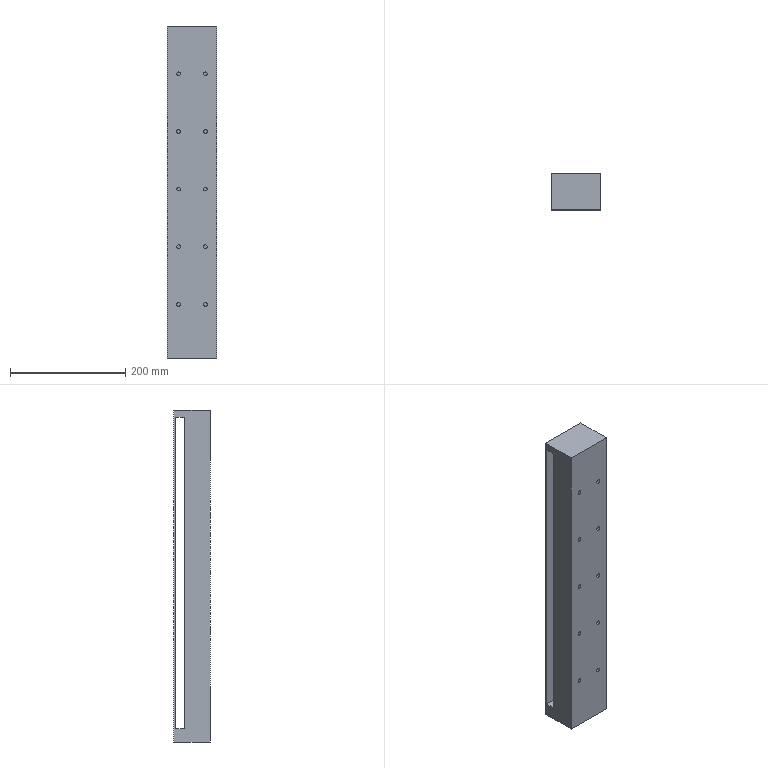Part | SolidWorks | features BaseBody 1 | 1 solid | 34 faces | box 86 x 63 x 576 mm | volume 613007 mm3 | cylinder 20 | plane 14 | commonest cylinder face diameters 6.5 x20
STEP:
#1=CARTESIAN_POINT('',(23.,-148.847,202.371));
#2=VERTEX_POINT('',#1);
#3=CARTESIAN_POINT('',(23.,-148.847,195.871));
#4=VERTEX_POINT('',#3);
#5=CARTESIAN_POINT('',(23.,-148.847,199.121));
#6=DIRECTION('',(0.,-1.,0.));
#7=DIRECTION('',(0.,0.,-1.));
#8=AXIS2_PLACEMENT_3D('',#5,#6,#7);
#9=CIRCLE('',#8,3.25);
#10=EDGE_CURVE('',#2,#4,#9,.T.);
#11=ORIENTED_EDGE('',*,*,#10,.F.);
#12=CARTESIAN_POINT('',(23.,-153.,202.371));
#13=VERTEX_POINT('',#12);
#14=CARTESIAN_POINT('',(23.,-133.,202.371));
#15=DIRECTION('',(0.,-1.,0.));
#16=VECTOR('',#15,1000.);
#17=LINE('',#14,#16);
#18=EDGE_CURVE('',#2,#13,#17,.T.);
#19=ORIENTED_EDGE('',*,*,#18,.T.);
#20=CARTESIAN_POINT('',(23.,-153.,195.871));
#21=VERTEX_POINT('',#20);
#22=CARTESIAN_POINT('',(23.,-153.,199.121));
#23=DIRECTION('',(0.,-1.,0.));
#24=DIRECTION('',(0.,0.,-1.));
#25=AXIS2_PLACEMENT_3D('',#22,#23,#24);
#26=CIRCLE('',#25,3.25);
#27=EDGE_CURVE('',#13,#21,#26,.T.);
#28=ORIENTED_EDGE('',*,*,#27,.T.);
#29=CARTESIAN_POINT('',(23.,-133.,195.871));
#30=DIRECTION('',(0.,-1.,0.));
#31=VECTOR('',#30,1000.);
#32=LINE('',#29,#31);
#33=EDGE_CURVE('',#4,#21,#32,.T.);
#34=ORIENTED_EDGE('',*,*,#33,.F.);
#35=EDGE_LOOP('',(#11,#19,#28,#34));
#36=FACE_OUTER_BOUND('',#35,.T.);
#37=CARTESIAN_POINT('',(23.,-133.,199.121));
#38=DIRECTION('',(0.,-1.,0.));
#39=DIRECTION('',(0.,0.,-1.));
#40=AXIS2_PLACEMENT_3D('',#37,#38,#39);
#41=CYLINDRICAL_SURFACE('',#40,3.25);
#42=ADVANCED_FACE('',(#36),#41,.F.);
#43=CARTESIAN_POINT('',(-23.,-148.847,202.371));
#44=VERTEX_POINT('',#43);
#45=CARTESIAN_POINT('',(-23.,-148.847,195.871));
#46=VERTEX_POINT('',#45);
#47=CARTESIAN_POINT('',(-23.,-148.847,199.121));
#48=DIRECTION('',(0.,-1.,0.));
#49=DIRECTION('',(0.,0.,-1.));
#50=AXIS2_PLACEMENT_3D('',#47,#48,#49);
#51=CIRCLE('',#50,3.25);
#52=EDGE_CURVE('',#44,#46,#51,.T.);
#53=ORIENTED_EDGE('',*,*,#52,.F.);
#54=CARTESIAN_POINT('',(-23.,-153.,202.371));
#55=VERTEX_POINT('',#54);
#56=CARTESIAN_POINT('',(-23.,-133.,202.371));
#57=DIRECTION('',(0.,-1.,0.));
#58=VECTOR('',#57,1000.);
#59=LINE('',#56,#58);
#60=EDGE_CURVE('',#44,#55,#59,.T.);
#61=ORIENTED_EDGE('',*,*,#60,.T.);
#62=CARTESIAN_POINT('',(-23.,-153.,195.871));
#63=VERTEX_POINT('',#62);
#64=CARTESIAN_POINT('',(-23.,-153.,199.121));
#65=DIRECTION('',(0.,-1.,0.));
#66=DIRECTION('',(0.,0.,-1.));
#67=AXIS2_PLACEMENT_3D('',#64,#65,#66);
#68=CIRCLE('',#67,3.25);
#69=EDGE_CURVE('',#55,#63,#68,.T.);
#70=ORIENTED_EDGE('',*,*,#69,.T.);
#71=CARTESIAN_POINT('',(-23.,-133.,195.871));
#72=DIRECTION('',(0.,-1.,0.));
#73=VECTOR('',#72,1000.);
#74=LINE('',#71,#73);
#75=EDGE_CURVE('',#46,#63,#74,.T.);
#76=ORIENTED_EDGE('',*,*,#75,.F.);
#77=EDGE_LOOP('',(#53,#61,#70,#76));
#78=FACE_OUTER_BOUND('',#77,.T.);
#79=CARTESIAN_POINT('',(-23.,-133.,199.121));
#80=DIRECTION('',(0.,-1.,0.));
#81=DIRECTION('',(0.,0.,-1.));
#82=AXIS2_PLACEMENT_3D('',#79,#80,#81);
#83=CYLINDRICAL_SURFACE('',#82,3.25);
#84=ADVANCED_FACE('',(#78),#83,.F.);
#85=CARTESIAN_POINT('',(23.,-148.847,102.371));
#86=VERTEX_POINT('',#85);
#87=CARTESIAN_POINT('',(23.,-148.847,95.871));
#88=VERTEX_POINT('',#87);
#89=CARTESIAN_POINT('',(23.,-148.847,99.121));
#90=DIRECTION('',(0.,-1.,0.));
#91=DIRECTION('',(0.,0.,-1.));
#92=AXIS2_PLACEMENT_3D('',#89,#90,#91);
#93=CIRCLE('',#92,3.25);
#94=EDGE_CURVE('',#86,#88,#93,.T.);
#95=ORIENTED_EDGE('',*,*,#94,.F.);
#96=CARTESIAN_POINT('',(23.,-153.,102.371));
#97=VERTEX_POINT('',#96);
#98=CARTESIAN_POINT('',(23.,-133.,102.371));
#99=DIRECTION('',(0.,-1.,0.));
#100=VECTOR('',#99,1000.);
#101=LINE('',#98,#100);
#102=EDGE_CURVE('',#86,#97,#101,.T.);
#103=ORIENTED_EDGE('',*,*,#102,.T.);
#104=CARTESIAN_POINT('',(23.,-153.,95.871));
#105=VERTEX_POINT('',#104);
#106=CARTESIAN_POINT('',(23.,-153.,99.121));
#107=DIRECTION('',(0.,-1.,0.));
#108=DIRECTION('',(0.,0.,-1.));
#109=AXIS2_PLACEMENT_3D('',#106,#107,#108);
#110=CIRCLE('',#109,3.25);
#111=EDGE_CURVE('',#97,#105,#110,.T.);
#112=ORIENTED_EDGE('',*,*,#111,.T.);
#113=CARTESIAN_POINT('',(23.,-133.,95.871));
#114=DIRECTION('',(0.,-1.,0.));
#115=VECTOR('',#114,1000.);
#116=LINE('',#113,#115);
#117=EDGE_CURVE('',#88,#105,#116,.T.);
#118=ORIENTED_EDGE('',*,*,#117,.F.);
#119=EDGE_LOOP('',(#95,#103,#112,#118));
#120=FACE_OUTER_BOUND('',#119,.T.);
#121=CARTESIAN_POINT('',(23.,-133.,99.121));
#122=DIRECTION('',(0.,-1.,0.));
#123=DIRECTION('',(0.,0.,-1.));
#124=AXIS2_PLACEMENT_3D('',#121,#122,#123);
#125=CYLINDRICAL_SURFACE('',#124,3.25);
#126=ADVANCED_FACE('',(#120),#125,.F.);
#127=CARTESIAN_POINT('',(-23.,-148.847,102.371));
#128=VERTEX_POINT('',#127);
#129=CARTESIAN_POINT('',(-23.,-148.847,95.871));
#130=VERTEX_POINT('',#129);
#131=CARTESIAN_POINT('',(-23.,-148.847,99.121));
#132=DIRECTION('',(0.,-1.,0.));
#133=DIRECTION('',(0.,0.,-1.));
#134=AXIS2_PLACEMENT_3D('',#131,#132,#133);
#135=CIRCLE('',#134,3.25);
#136=EDGE_CURVE('',#128,#130,#135,.T.);
#137=ORIENTED_EDGE('',*,*,#136,.F.);
#138=CARTESIAN_POINT('',(-23.,-153.,102.371));
#139=VERTEX_POINT('',#138);
#140=CARTESIAN_POINT('',(-23.,-133.,102.371));
#141=DIRECTION('',(0.,-1.,0.));
#142=VECTOR('',#141,1000.);
#143=LINE('',#140,#142);
#144=EDGE_CURVE('',#128,#139,#143,.T.);
#145=ORIENTED_EDGE('',*,*,#144,.T.);
#146=CARTESIAN_POINT('',(-23.,-153.,95.871));
#147=VERTEX_POINT('',#146);
#148=CARTESIAN_POINT('',(-23.,-153.,99.121));
#149=DIRECTION('',(0.,-1.,0.));
#150=DIRECTION('',(0.,0.,-1.));
#151=AXIS2_PLACEMENT_3D('',#148,#149,#150);
#152=CIRCLE('',#151,3.25);
#153=EDGE_CURVE('',#139,#147,#152,.T.);
#154=ORIENTED_EDGE('',*,*,#153,.T.);
#155=CARTESIAN_POINT('',(-23.,-133.,95.871));
#156=DIRECTION('',(0.,-1.,0.));
#157=VECTOR('',#156,1000.);
#158=LINE('',#155,#157);
#159=EDGE_CURVE('',#130,#147,#158,.T.);
#160=ORIENTED_EDGE('',*,*,#159,.F.);
#161=EDGE_LOOP('',(#137,#145,#154,#160));
#162=FACE_OUTER_BOUND('',#161,.T.);
#163=CARTESIAN_POINT('',(-23.,-133.,99.121));
#164=DIRECTION('',(0.,-1.,0.));
#165=DIRECTION('',(0.,0.,-1.));
#166=AXIS2_PLACEMENT_3D('',#163,#164,#165);
#167=CYLINDRICAL_SURFACE('',#166,3.25);
#168=ADVANCED_FACE('',(#162),#167,.F.);
#169=CARTESIAN_POINT('',(23.,-148.847,2.371));
#170=VERTEX_POINT('',#169);
#171=CARTESIAN_POINT('',(23.,-148.847,-4.129));
#172=VERTEX_POINT('',#171);
#173=CARTESIAN_POINT('',(23.,-148.847,-0.8789));
#174=DIRECTION('',(0.,-1.,0.));
#175=DIRECTION('',(0.,0.,-1.));
#176=AXIS2_PLACEMENT_3D('',#173,#174,#175);
#177=CIRCLE('',#176,3.25);
#178=EDGE_CURVE('',#170,#172,#177,.T.);
#179=ORIENTED_EDGE('',*,*,#178,.F.);
#180=CARTESIAN_POINT('',(23.,-153.,2.371));
#181=VERTEX_POINT('',#180);
#182=CARTESIAN_POINT('',(23.,-133.,2.371));
#183=DIRECTION('',(0.,-1.,0.));
#184=VECTOR('',#183,1000.);
#185=LINE('',#182,#184);
#186=EDGE_CURVE('',#170,#181,#185,.T.);
#187=ORIENTED_EDGE('',*,*,#186,.T.);
#188=CARTESIAN_POINT('',(23.,-153.,-4.129));
#189=VERTEX_POINT('',#188);
#190=CARTESIAN_POINT('',(23.,-153.,-0.8789));
#191=DIRECTION('',(0.,-1.,0.));
#192=DIRECTION('',(0.,0.,-1.));
#193=AXIS2_PLACEMENT_3D('',#190,#191,#192);
#194=CIRCLE('',#193,3.25);
#195=EDGE_CURVE('',#181,#189,#194,.T.);
#196=ORIENTED_EDGE('',*,*,#195,.T.);
#197=CARTESIAN_POINT('',(23.,-133.,-4.129));
#198=DIRECTION('',(0.,-1.,0.));
#199=VECTOR('',#198,1000.);
#200=LINE('',#197,#199);
#201=EDGE_CURVE('',#172,#189,#200,.T.);
#202=ORIENTED_EDGE('',*,*,#201,.F.);
#203=EDGE_LOOP('',(#179,#187,#196,#202));
#204=FACE_OUTER_BOUND('',#203,.T.);
#205=CARTESIAN_POINT('',(23.,-133.,-0.8789));
#206=DIRECTION('',(0.,-1.,0.));
#207=DIRECTION('',(0.,0.,-1.));
#208=AXIS2_PLACEMENT_3D('',#205,#206,#207);
#209=CYLINDRICAL_SURFACE('',#208,3.25);
#210=ADVANCED_FACE('',(#204),#209,.F.);
#211=CARTESIAN_POINT('',(-23.,-148.847,2.371));
#212=VERTEX_POINT('',#211);
#213=CARTESIAN_POINT('',(-23.,-148.847,-4.129));
#214=VERTEX_POINT('',#213);
#215=CARTESIAN_POINT('',(-23.,-148.847,-0.8789));
#216=DIRECTION('',(0.,-1.,0.));
#217=DIRECTION('',(0.,0.,-1.));
#218=AXIS2_PLACEMENT_3D('',#215,#216,#217);
#219=CIRCLE('',#218,3.25);
#220=EDGE_CURVE('',#212,#214,#219,.T.);
#221=ORIENTED_EDGE('',*,*,#220,.F.);
#222=CARTESIAN_POINT('',(-23.,-153.,2.371));
#223=VERTEX_POINT('',#222);
#224=CARTESIAN_POINT('',(-23.,-133.,2.371));
#225=DIRECTION('',(0.,-1.,0.));
#226=VECTOR('',#225,1000.);
#227=LINE('',#224,#226);
#228=EDGE_CURVE('',#212,#223,#227,.T.);
#229=ORIENTED_EDGE('',*,*,#228,.T.);
#230=CARTESIAN_POINT('',(-23.,-153.,-4.129));
#231=VERTEX_POINT('',#230);
#232=CARTESIAN_POINT('',(-23.,-153.,-0.8789));
#233=DIRECTION('',(0.,-1.,0.));
#234=DIRECTION('',(0.,0.,-1.));
#235=AXIS2_PLACEMENT_3D('',#232,#233,#234);
#236=CIRCLE('',#235,3.25);
#237=EDGE_CURVE('',#223,#231,#236,.T.);
#238=ORIENTED_EDGE('',*,*,#237,.T.);
#239=CARTESIAN_POINT('',(-23.,-133.,-4.129));
#240=DIRECTION('',(0.,-1.,0.));
#241=VECTOR('',#240,1000.);
#242=LINE('',#239,#241);
#243=EDGE_CURVE('',#214,#231,#242,.T.);
#244=ORIENTED_EDGE('',*,*,#243,.F.);
#245=EDGE_LOOP('',(#221,#229,#238,#244));
#246=FACE_OUTER_BOUND('',#245,.T.);
#247=CARTESIAN_POINT('',(-23.,-133.,-0.8789));
#248=DIRECTION('',(0.,-1.,0.));
#249=DIRECTION('',(0.,0.,-1.));
#250=AXIS2_PLACEMENT_3D('',#247,#248,#249);
#251=CYLINDRICAL_SURFACE('',#250,3.25);
#252=ADVANCED_FACE('',(#246),#251,.F.);
#253=CARTESIAN_POINT('',(23.,-148.847,-97.629));
#254=VERTEX_POINT('',#253);
#255=CARTESIAN_POINT('',(23.,-148.847,-104.129));
#256=VERTEX_POINT('',#255);
#257=CARTESIAN_POINT('',(23.,-148.847,-100.879));
#258=DIRECTION('',(0.,-1.,0.));
#259=DIRECTION('',(0.,0.,-1.));
#260=AXIS2_PLACEMENT_3D('',#257,#258,#259);
#261=CIRCLE('',#260,3.25);
#262=EDGE_CURVE('',#254,#256,#261,.T.);
#263=ORIENTED_EDGE('',*,*,#262,.F.);
#264=CARTESIAN_POINT('',(23.,-153.,-97.629));
#265=VERTEX_POINT('',#264);
#266=CARTESIAN_POINT('',(23.,-133.,-97.629));
#267=DIRECTION('',(0.,-1.,0.));
#268=VECTOR('',#267,1000.);
#269=LINE('',#266,#268);
#270=EDGE_CURVE('',#254,#265,#269,.T.);
#271=ORIENTED_EDGE('',*,*,#270,.T.);
#272=CARTESIAN_POINT('',(23.,-153.,-104.129));
#273=VERTEX_POINT('',#272);
#274=CARTESIAN_POINT('',(23.,-153.,-100.879));
#275=DIRECTION('',(0.,-1.,0.));
#276=DIRECTION('',(0.,0.,-1.));
#277=AXIS2_PLACEMENT_3D('',#274,#275,#276);
#278=CIRCLE('',#277,3.25);
#279=EDGE_CURVE('',#265,#273,#278,.T.);
#280=ORIENTED_EDGE('',*,*,#279,.T.);
#281=CARTESIAN_POINT('',(23.,-133.,-104.129));
#282=DIRECTION('',(0.,-1.,0.));
#283=VECTOR('',#282,1000.);
#284=LINE('',#281,#283);
#285=EDGE_CURVE('',#256,#273,#284,.T.);
#286=ORIENTED_EDGE('',*,*,#285,.F.);
#287=EDGE_LOOP('',(#263,#271,#280,#286));
#288=FACE_OUTER_BOUND('',#287,.T.);
#289=CARTESIAN_POINT('',(23.,-133.,-100.879));
#290=DIRECTION('',(0.,-1.,0.));
#291=DIRECTION('',(0.,0.,-1.));
#292=AXIS2_PLACEMENT_3D('',#289,#290,#291);
#293=CYLINDRICAL_SURFACE('',#292,3.25);
#294=ADVANCED_FACE('',(#288),#293,.F.);
#295=CARTESIAN_POINT('',(-23.,-148.847,-97.629));
#296=VERTEX_POINT('',#295);
#297=CARTESIAN_POINT('',(-23.,-148.847,-104.129));
#298=VERTEX_POINT('',#297);
#299=CARTESIAN_POINT('',(-23.,-148.847,-100.879));
#300=DIRECTION('',(0.,-1.,0.));
#301=DIRECTION('',(0.,0.,-1.));
#302=AXIS2_PLACEMENT_3D('',#299,#300,#301);
#303=CIRCLE('',#302,3.25);
#304=EDGE_CURVE('',#296,#298,#303,.T.);
#305=ORIENTED_EDGE('',*,*,#304,.F.);
#306=CARTESIAN_POINT('',(-23.,-153.,-97.629));
#307=VERTEX_POINT('',#306);
#308=CARTESIAN_POINT('',(-23.,-133.,-97.629));
#309=DIRECTION('',(0.,-1.,0.));
#310=VECTOR('',#309,1000.);
#311=LINE('',#308,#310);
#312=EDGE_CURVE('',#296,#307,#311,.T.);
#313=ORIENTED_EDGE('',*,*,#312,.T.);
#314=CARTESIAN_POINT('',(-23.,-153.,-104.129));
#315=VERTEX_POINT('',#314);
#316=CARTESIAN_POINT('',(-23.,-153.,-100.879));
#317=DIRECTION('',(0.,-1.,0.));
#318=DIRECTION('',(0.,0.,-1.));
#319=AXIS2_PLACEMENT_3D('',#316,#317,#318);
#320=CIRCLE('',#319,3.25);
#321=EDGE_CURVE('',#307,#315,#320,.T.);
#322=ORIENTED_EDGE('',*,*,#321,.T.);
#323=CARTESIAN_POINT('',(-23.,-133.,-104.129));
#324=DIRECTION('',(0.,-1.,0.));
#325=VECTOR('',#324,1000.);
#326=LINE('',#323,#325);
#327=EDGE_CURVE('',#298,#315,#326,.T.);
#328=ORIENTED_EDGE('',*,*,#327,.F.);
#329=EDGE_LOOP('',(#305,#313,#322,#328));
#330=FACE_OUTER_BOUND('',#329,.T.);
#331=CARTESIAN_POINT('',(-23.,-133.,-100.879));
#332=DIRECTION('',(0.,-1.,0.));
#333=DIRECTION('',(0.,0.,-1.));
#334=AXIS2_PLACEMENT_3D('',#331,#332,#333);
#335=CYLINDRICAL_SURFACE('',#334,3.25);
#336=ADVANCED_FACE('',(#330),#335,.F.);
#337=CARTESIAN_POINT('',(23.,-148.847,-197.629));
#338=VERTEX_POINT('',#337);
#339=CARTESIAN_POINT('',(23.,-148.847,-204.129));
#340=VERTEX_POINT('',#339);
#341=CARTESIAN_POINT('',(23.,-148.847,-200.879));
#342=DIRECTION('',(0.,-1.,0.));
#343=DIRECTION('',(0.,0.,-1.));
#344=AXIS2_PLACEMENT_3D('',#341,#342,#343);
#345=CIRCLE('',#344,3.25);
#346=EDGE_CURVE('',#338,#340,#345,.T.);
#347=ORIENTED_EDGE('',*,*,#346,.F.);
#348=CARTESIAN_POINT('',(23.,-153.,-197.629));
#349=VERTEX_POINT('',#348);
#350=CARTESIAN_POINT('',(23.,-133.,-197.629));
#351=DIRECTION('',(0.,-1.,0.));
#352=VECTOR('',#351,1000.);
#353=LINE('',#350,#352);
#354=EDGE_CURVE('',#338,#349,#353,.T.);
#355=ORIENTED_EDGE('',*,*,#354,.T.);
#356=CARTESIAN_POINT('',(23.,-153.,-204.129));
#357=VERTEX_POINT('',#356);
#358=CARTESIAN_POINT('',(23.,-153.,-200.879));
#359=DIRECTION('',(0.,-1.,0.));
#360=DIRECTION('',(0.,0.,-1.));
#361=AXIS2_PLACEMENT_3D('',#358,#359,#360);
#362=CIRCLE('',#361,3.25);
#363=EDGE_CURVE('',#349,#357,#362,.T.);
#364=ORIENTED_EDGE('',*,*,#363,.T.);
#365=CARTESIAN_POINT('',(23.,-133.,-204.129));
#366=DIRECTION('',(0.,-1.,0.));
#367=VECTOR('',#366,1000.);
#368=LINE('',#365,#367);
#369=EDGE_CURVE('',#340,#357,#368,.T.);
#370=ORIENTED_EDGE('',*,*,#369,.F.);
#371=EDGE_LOOP('',(#347,#355,#364,#370));
#372=FACE_OUTER_BOUND('',#371,.T.);
#373=CARTESIAN_POINT('',(23.,-133.,-200.879));
#374=DIRECTION('',(0.,-1.,0.));
#375=DIRECTION('',(0.,0.,-1.));
#376=AXIS2_PLACEMENT_3D('',#373,#374,#375);
#377=CYLINDRICAL_SURFACE('',#376,3.25);
#378=ADVANCED_FACE('',(#372),#377,.F.);
#379=CARTESIAN_POINT('',(-23.,-148.847,-197.629));
#380=VERTEX_POINT('',#379);
#381=CARTESIAN_POINT('',(-23.,-148.847,-204.129));
#382=VERTEX_POINT('',#381);
#383=CARTESIAN_POINT('',(-23.,-148.847,-200.879));
#384=DIRECTION('',(0.,-1.,0.));
#385=DIRECTION('',(0.,0.,-1.));
#386=AXIS2_PLACEMENT_3D('',#383,#384,#385);
#387=CIRCLE('',#386,3.25);
#388=EDGE_CURVE('',#380,#382,#387,.T.);
#389=ORIENTED_EDGE('',*,*,#388,.F.);
#390=CARTESIAN_POINT('',(-23.,-153.,-197.629));
#391=VERTEX_POINT('',#390);
#392=CARTESIAN_POINT('',(-23.,-133.,-197.629));
#393=DIRECTION('',(0.,-1.,0.));
#394=VECTOR('',#393,1000.);
#395=LINE('',#392,#394);
#396=EDGE_CURVE('',#380,#391,#395,.T.);
#397=ORIENTED_EDGE('',*,*,#396,.T.);
#398=CARTESIAN_POINT('',(-23.,-153.,-204.129));
#399=VERTEX_POINT('',#398);
#400=CARTESIAN_POINT('',(-23.,-153.,-200.879));
#401=DIRECTION('',(0.,-1.,0.));
#402=DIRECTION('',(0.,0.,-1.));
#403=AXIS2_PLACEMENT_3D('',#400,#401,#402);
#404=CIRCLE('',#403,3.25);
#405=EDGE_CURVE('',#391,#399,#404,.T.);
#406=ORIENTED_EDGE('',*,*,#405,.T.);
#407=CARTESIAN_POINT('',(-23.,-133.,-204.129));
#408=DIRECTION('',(0.,-1.,0.));
#409=VECTOR('',#408,1000.);
#410=LINE('',#407,#409);
#411=EDGE_CURVE('',#382,#399,#410,.T.);
#412=ORIENTED_EDGE('',*,*,#411,.F.);
#413=EDGE_LOOP('',(#389,#397,#406,#412));
#414=FACE_OUTER_BOUND('',#413,.T.);
#415=CARTESIAN_POINT('',(-23.,-133.,-200.879));
#416=DIRECTION('',(0.,-1.,0.));
#417=DIRECTION('',(0.,0.,-1.));
#418=AXIS2_PLACEMENT_3D('',#415,#416,#417);
#419=CYLINDRICAL_SURFACE('',#418,3.25);
#420=ADVANCED_FACE('',(#414),#419,.F.);
#421=CARTESIAN_POINT('',(-43.,-90.,282.121));
#422=VERTEX_POINT('',#421);
#423=CARTESIAN_POINT('',(-43.,-90.,-293.879));
#424=VERTEX_POINT('',#423);
#425=CARTESIAN_POINT('',(-43.,-90.,282.121));
#426=DIRECTION('',(0.,0.,-1.));
#427=VECTOR('',#426,1000.);
#428=LINE('',#425,#427);
#429=EDGE_CURVE('',#422,#424,#428,.T.);
#430=ORIENTED_EDGE('',*,*,#429,.F.);
#431=CARTESIAN_POINT('',(43.,-90.,282.121));
#432=VERTEX_POINT('',#431);
#433=CARTESIAN_POINT('',(-43.,-90.,282.121));
#434=DIRECTION('',(-1.,0.,0.));
#435=VECTOR('',#434,1000.);
#436=LINE('',#433,#435);
#437=EDGE_CURVE('',#432,#422,#436,.T.);
#438=ORIENTED_EDGE('',*,*,#437,.F.);
#439=CARTESIAN_POINT('',(43.,-90.,-293.879));
#440=VERTEX_POINT('',#439);
#441=CARTESIAN_POINT('',(43.,-90.,282.121));
#442=DIRECTION('',(0.,0.,1.));
#443=VECTOR('',#442,1000.);
#444=LINE('',#441,#443);
#445=EDGE_CURVE('',#440,#432,#444,.T.);
#446=ORIENTED_EDGE('',*,*,#445,.F.);
#447=CARTESIAN_POINT('',(-43.,-90.,-293.879));
#448=DIRECTION('',(1.,0.,0.));
#449=VECTOR('',#448,1000.);
#450=LINE('',#447,#449);
#451=EDGE_CURVE('',#424,#440,#450,.T.);
#452=ORIENTED_EDGE('',*,*,#451,.F.);
#453=EDGE_LOOP('',(#430,#438,#446,#452));
#454=FACE_OUTER_BOUND('',#453,.T.);
#455=CARTESIAN_POINT('',(-43.,-90.,282.121));
#456=DIRECTION('',(0.,-1.,0.));
#457=DIRECTION('',(0.,0.,-1.));
#458=AXIS2_PLACEMENT_3D('',#455,#456,#457);
#459=PLANE('',#458);
#460=ADVANCED_FACE('',(#454),#459,.F.);
#461=CARTESIAN_POINT('',(-43.,-153.,-293.879));
#462=VERTEX_POINT('',#461);
#463=CARTESIAN_POINT('',(43.,-153.,-293.879));
#464=VERTEX_POINT('',#463);
#465=CARTESIAN_POINT('',(0.,-153.,-293.879));
#466=DIRECTION('',(1.,0.,0.));
#467=VECTOR('',#466,1000.);
#468=LINE('',#465,#467);
#469=EDGE_CURVE('',#462,#464,#468,.T.);
#470=ORIENTED_EDGE('',*,*,#469,.F.);
#471=CARTESIAN_POINT('',(-43.,-121.5,-293.879));
#472=DIRECTION('',(0.,-1.,0.));
#473=VECTOR('',#472,1000.);
#474=LINE('',#471,#473);
#475=EDGE_CURVE('',#424,#462,#474,.T.);
#476=ORIENTED_EDGE('',*,*,#475,.F.);
#477=ORIENTED_EDGE('',*,*,#451,.T.);
#478=CARTESIAN_POINT('',(43.,-121.5,-293.879));
#479=DIRECTION('',(0.,1.,0.));
#480=VECTOR('',#479,1000.);
#481=LINE('',#478,#480);
#482=EDGE_CURVE('',#464,#440,#481,.T.);
#483=ORIENTED_EDGE('',*,*,#482,.F.);
#484=EDGE_LOOP('',(#470,#476,#477,#483));
#485=FACE_OUTER_BOUND('',#484,.T.);
#486=CARTESIAN_POINT('',(0.,-121.5,-293.879));
#487=DIRECTION('',(0.,0.,1.));
#488=DIRECTION('',(1.,0.,0.));
#489=AXIS2_PLACEMENT_3D('',#486,#487,#488);
#490=PLANE('',#489);
#491=ADVANCED_FACE('',(#485),#490,.F.);
#492=CARTESIAN_POINT('',(-43.,-93.,269.121));
#493=VERTEX_POINT('',#492);
#494=CARTESIAN_POINT('',(-43.,-93.,-270.879));
#495=VERTEX_POINT('',#494);
#496=CARTESIAN_POINT('',(-43.,-93.,282.121));
#497=DIRECTION('',(0.,0.,-1.));
#498=VECTOR('',#497,1000.);
#499=LINE('',#496,#498);
#500=EDGE_CURVE('',#493,#495,#499,.T.);
#501=ORIENTED_EDGE('',*,*,#500,.F.);
#502=CARTESIAN_POINT('',(-43.,-108.5,269.121));
#503=VERTEX_POINT('',#502);
#504=CARTESIAN_POINT('',(-43.,-90.,269.121));
#505=DIRECTION('',(0.,1.,0.));
#506=VECTOR('',#505,1000.);
#507=LINE('',#504,#506);
#508=EDGE_CURVE('',#503,#493,#507,.T.);
#509=ORIENTED_EDGE('',*,*,#508,.F.);
#510=CARTESIAN_POINT('',(-43.,-108.5,-270.879));
#511=VERTEX_POINT('',#510);
#512=CARTESIAN_POINT('',(-43.,-108.5,282.121));
#513=DIRECTION('',(0.,0.,1.));
#514=VECTOR('',#513,1000.);
#515=LINE('',#512,#514);
#516=EDGE_CURVE('',#511,#503,#515,.T.);
#517=ORIENTED_EDGE('',*,*,#516,.F.);
#518=CARTESIAN_POINT('',(-43.,-90.,-270.879));
#519=DIRECTION('',(0.,-1.,0.));
#520=VECTOR('',#519,1000.);
#521=LINE('',#518,#520);
#522=EDGE_CURVE('',#495,#511,#521,.T.);
#523=ORIENTED_EDGE('',*,*,#522,.F.);
#524=EDGE_LOOP('',(#501,#509,#517,#523));
#525=FACE_BOUND('',#524,.T.);
#526=CARTESIAN_POINT('',(-43.,-153.,282.121));
#527=VERTEX_POINT('',#526);
#528=CARTESIAN_POINT('',(-43.,-153.,282.121));
#529=DIRECTION('',(0.,0.,-1.));
#530=VECTOR('',#529,1000.);
#531=LINE('',#528,#530);
#532=EDGE_CURVE('',#527,#462,#531,.T.);
#533=ORIENTED_EDGE('',*,*,#532,.F.);
#534=CARTESIAN_POINT('',(-43.,-90.,282.121));
#535=DIRECTION('',(0.,-1.,0.));
#536=VECTOR('',#535,1000.);
#537=LINE('',#534,#536);
#538=EDGE_CURVE('',#422,#527,#537,.T.);
#539=ORIENTED_EDGE('',*,*,#538,.F.);
#540=ORIENTED_EDGE('',*,*,#429,.T.);
#541=ORIENTED_EDGE('',*,*,#475,.T.);
#542=EDGE_LOOP('',(#533,#539,#540,#541));
#543=FACE_OUTER_BOUND('',#542,.T.);
#544=CARTESIAN_POINT('',(-43.,-90.,282.121));
#545=DIRECTION('',(1.,0.,0.));
#546=DIRECTION('',(0.,0.,-1.));
#547=AXIS2_PLACEMENT_3D('',#544,#545,#546);
#548=PLANE('',#547);
#549=ADVANCED_FACE('',(#525,#543),#548,.F.);
#550=ORIENTED_EDGE('',*,*,#538,.T.);
#551=CARTESIAN_POINT('',(43.,-153.,282.121));
#552=VERTEX_POINT('',#551);
#553=CARTESIAN_POINT('',(0.,-153.,282.121));
#554=DIRECTION('',(1.,0.,0.));
#555=VECTOR('',#554,1000.);
#556=LINE('',#553,#555);
#557=EDGE_CURVE('',#527,#552,#556,.T.);
#558=ORIENTED_EDGE('',*,*,#557,.T.);
#559=CARTESIAN_POINT('',(43.,-121.5,282.121));
#560=DIRECTION('',(0.,1.,0.));
#561=VECTOR('',#560,1000.);
#562=LINE('',#559,#561);
#563=EDGE_CURVE('',#552,#432,#562,.T.);
#564=ORIENTED_EDGE('',*,*,#563,.T.);
#565=ORIENTED_EDGE('',*,*,#437,.T.);
#566=EDGE_LOOP('',(#550,#558,#564,#565));
#567=FACE_OUTER_BOUND('',#566,.T.);
#568=CARTESIAN_POINT('',(0.,-121.5,282.121));
#569=DIRECTION('',(0.,0.,1.));
#570=DIRECTION('',(1.,0.,0.));
#571=AXIS2_PLACEMENT_3D('',#568,#569,#570);
#572=PLANE('',#571);
#573=ADVANCED_FACE('',(#567),#572,.T.);
#574=CARTESIAN_POINT('',(43.,-108.5,269.121));
#575=VERTEX_POINT('',#574);
#576=CARTESIAN_POINT('',(43.,-108.5,-270.879));
#577=VERTEX_POINT('',#576);
#578=CARTESIAN_POINT('',(43.,-108.5,282.121));
#579=DIRECTION('',(0.,0.,-1.));
#580=VECTOR('',#579,1000.);
#581=LINE('',#578,#580);
#582=EDGE_CURVE('',#575,#577,#581,.T.);
#583=ORIENTED_EDGE('',*,*,#582,.F.);
#584=CARTESIAN_POINT('',(43.,-93.,269.121));
#585=VERTEX_POINT('',#584);
#586=CARTESIAN_POINT('',(43.,-90.,269.121));
#587=DIRECTION('',(0.,-1.,0.));
#588=VECTOR('',#587,1000.);
#589=LINE('',#586,#588);
#590=EDGE_CURVE('',#585,#575,#589,.T.);
#591=ORIENTED_EDGE('',*,*,#590,.F.);
#592=CARTESIAN_POINT('',(43.,-93.,-270.879));
#593=VERTEX_POINT('',#592);
#594=CARTESIAN_POINT('',(43.,-93.,282.121));
#595=DIRECTION('',(0.,0.,1.));
#596=VECTOR('',#595,1000.);
#597=LINE('',#594,#596);
#598=EDGE_CURVE('',#593,#585,#597,.T.);
#599=ORIENTED_EDGE('',*,*,#598,.F.);
#600=CARTESIAN_POINT('',(43.,-90.,-270.879));
#601=DIRECTION('',(0.,1.,0.));
#602=VECTOR('',#601,1000.);
#603=LINE('',#600,#602);
#604=EDGE_CURVE('',#577,#593,#603,.T.);
#605=ORIENTED_EDGE('',*,*,#604,.F.);
#606=EDGE_LOOP('',(#583,#591,#599,#605));
#607=FACE_BOUND('',#606,.T.);
#608=ORIENTED_EDGE('',*,*,#445,.T.);
#609=ORIENTED_EDGE('',*,*,#563,.F.);
#610=CARTESIAN_POINT('',(43.,-153.,282.121));
#611=DIRECTION('',(0.,0.,1.));
#612=VECTOR('',#611,1000.);
#613=LINE('',#610,#612);
#614=EDGE_CURVE('',#464,#552,#613,.T.);
#615=ORIENTED_EDGE('',*,*,#614,.F.);
#616=ORIENTED_EDGE('',*,*,#482,.T.);
#617=EDGE_LOOP('',(#608,#609,#615,#616));
#618=FACE_OUTER_BOUND('',#617,.T.);
#619=CARTESIAN_POINT('',(43.,-90.,282.121));
#620=DIRECTION('',(-1.,0.,0.));
#621=DIRECTION('',(0.,0.,1.));
#622=AXIS2_PLACEMENT_3D('',#619,#620,#621);
#623=PLANE('',#622);
#624=ADVANCED_FACE('',(#607,#618),#623,.F.);
#625=ORIENTED_EDGE('',*,*,#614,.T.);
#626=ORIENTED_EDGE('',*,*,#557,.F.);
#627=ORIENTED_EDGE('',*,*,#532,.T.);
#628=ORIENTED_EDGE('',*,*,#469,.T.);
#629=EDGE_LOOP('',(#625,#626,#627,#628));
#630=FACE_OUTER_BOUND('',#629,.T.);
#631=CARTESIAN_POINT('',(23.,-153.,199.121));
#632=DIRECTION('',(0.,-1.,0.));
#633=DIRECTION('',(0.,0.,-1.));
#634=AXIS2_PLACEMENT_3D('',#631,#632,#633);
#635=CIRCLE('',#634,3.25);
#636=EDGE_CURVE('',#21,#13,#635,.T.);
#637=ORIENTED_EDGE('',*,*,#636,.F.);
#638=ORIENTED_EDGE('',*,*,#27,.F.);
#639=EDGE_LOOP('',(#637,#638));
#640=FACE_BOUND('',#639,.T.);
#641=CARTESIAN_POINT('',(-23.,-153.,199.121));
#642=DIRECTION('',(0.,-1.,0.));
#643=DIRECTION('',(0.,0.,-1.));
#644=AXIS2_PLACEMENT_3D('',#641,#642,#643);
#645=CIRCLE('',#644,3.25);
#646=EDGE_CURVE('',#63,#55,#645,.T.);
#647=ORIENTED_EDGE('',*,*,#646,.F.);
#648=ORIENTED_EDGE('',*,*,#69,.F.);
#649=EDGE_LOOP('',(#647,#648));
#650=FACE_BOUND('',#649,.T.);
#651=CARTESIAN_POINT('',(23.,-153.,99.121));
#652=DIRECTION('',(0.,-1.,0.));
#653=DIRECTION('',(0.,0.,-1.));
#654=AXIS2_PLACEMENT_3D('',#651,#652,#653);
#655=CIRCLE('',#654,3.25);
#656=EDGE_CURVE('',#105,#97,#655,.T.);
#657=ORIENTED_EDGE('',*,*,#656,.F.);
#658=ORIENTED_EDGE('',*,*,#111,.F.);
#659=EDGE_LOOP('',(#657,#658));
#660=FACE_BOUND('',#659,.T.);
#661=CARTESIAN_POINT('',(-23.,-153.,99.121));
#662=DIRECTION('',(0.,-1.,0.));
#663=DIRECTION('',(0.,0.,-1.));
#664=AXIS2_PLACEMENT_3D('',#661,#662,#663);
#665=CIRCLE('',#664,3.25);
#666=EDGE_CURVE('',#147,#139,#665,.T.);
#667=ORIENTED_EDGE('',*,*,#666,.F.);
#668=ORIENTED_EDGE('',*,*,#153,.F.);
#669=EDGE_LOOP('',(#667,#668));
#670=FACE_BOUND('',#669,.T.);
#671=CARTESIAN_POINT('',(23.,-153.,-0.8789));
#672=DIRECTION('',(0.,-1.,0.));
#673=DIRECTION('',(0.,0.,-1.));
#674=AXIS2_PLACEMENT_3D('',#671,#672,#673);
#675=CIRCLE('',#674,3.25);
#676=EDGE_CURVE('',#189,#181,#675,.T.);
#677=ORIENTED_EDGE('',*,*,#676,.F.);
#678=ORIENTED_EDGE('',*,*,#195,.F.);
#679=EDGE_LOOP('',(#677,#678));
#680=FACE_BOUND('',#679,.T.);
#681=CARTESIAN_POINT('',(-23.,-153.,-0.8789));
#682=DIRECTION('',(0.,-1.,0.));
#683=DIRECTION('',(0.,0.,-1.));
#684=AXIS2_PLACEMENT_3D('',#681,#682,#683);
#685=CIRCLE('',#684,3.25);
#686=EDGE_CURVE('',#231,#223,#685,.T.);
#687=ORIENTED_EDGE('',*,*,#686,.F.);
#688=ORIENTED_EDGE('',*,*,#237,.F.);
#689=EDGE_LOOP('',(#687,#688));
#690=FACE_BOUND('',#689,.T.);
#691=CARTESIAN_POINT('',(23.,-153.,-100.879));
#692=DIRECTION('',(0.,-1.,0.));
#693=DIRECTION('',(0.,0.,-1.));
#694=AXIS2_PLACEMENT_3D('',#691,#692,#693);
#695=CIRCLE('',#694,3.25);
#696=EDGE_CURVE('',#273,#265,#695,.T.);
#697=ORIENTED_EDGE('',*,*,#696,.F.);
#698=ORIENTED_EDGE('',*,*,#279,.F.);
#699=EDGE_LOOP('',(#697,#698));
#700=FACE_BOUND('',#699,.T.);
#701=CARTESIAN_POINT('',(-23.,-153.,-100.879));
#702=DIRECTION('',(0.,-1.,0.));
#703=DIRECTION('',(0.,0.,-1.));
#704=AXIS2_PLACEMENT_3D('',#701,#702,#703);
#705=CIRCLE('',#704,3.25);
#706=EDGE_CURVE('',#315,#307,#705,.T.);
#707=ORIENTED_EDGE('',*,*,#706,.F.);
#708=ORIENTED_EDGE('',*,*,#321,.F.);
#709=EDGE_LOOP('',(#707,#708));
#710=FACE_BOUND('',#709,.T.);
#711=CARTESIAN_POINT('',(23.,-153.,-200.879));
#712=DIRECTION('',(0.,-1.,0.));
#713=DIRECTION('',(0.,0.,-1.));
#714=AXIS2_PLACEMENT_3D('',#711,#712,#713);
#715=CIRCLE('',#714,3.25);
#716=EDGE_CURVE('',#357,#349,#715,.T.);
#717=ORIENTED_EDGE('',*,*,#716,.F.);
#718=ORIENTED_EDGE('',*,*,#363,.F.);
#719=EDGE_LOOP('',(#717,#718));
#720=FACE_BOUND('',#719,.T.);
#721=CARTESIAN_POINT('',(-23.,-153.,-200.879));
#722=DIRECTION('',(0.,-1.,0.));
#723=DIRECTION('',(0.,0.,-1.));
#724=AXIS2_PLACEMENT_3D('',#721,#722,#723);
#725=CIRCLE('',#724,3.25);
#726=EDGE_CURVE('',#399,#391,#725,.T.);
#727=ORIENTED_EDGE('',*,*,#726,.F.);
#728=ORIENTED_EDGE('',*,*,#405,.F.);
#729=EDGE_LOOP('',(#727,#728));
#730=FACE_BOUND('',#729,.T.);
#731=CARTESIAN_POINT('',(-43.,-153.,282.121));
#732=DIRECTION('',(0.,1.,0.));
#733=DIRECTION('',(0.,0.,1.));
#734=AXIS2_PLACEMENT_3D('',#731,#732,#733);
#735=PLANE('',#734);
#736=ADVANCED_FACE('',(#630,#640,#650,#660,#670,#680,#690,#700,#710,#720,#730),#735,.F.);
#737=ORIENTED_EDGE('',*,*,#604,.T.);
#738=CARTESIAN_POINT('',(0.,-93.,-270.879));
#739=DIRECTION('',(-1.,0.,0.));
#740=VECTOR('',#739,1000.);
#741=LINE('',#738,#740);
#742=EDGE_CURVE('',#593,#495,#741,.T.);
#743=ORIENTED_EDGE('',*,*,#742,.T.);
#744=ORIENTED_EDGE('',*,*,#522,.T.);
#745=CARTESIAN_POINT('',(-41.,-108.5,-270.879));
#746=VERTEX_POINT('',#745);
#747=CARTESIAN_POINT('',(0.,-108.5,-270.879));
#748=DIRECTION('',(1.,0.,0.));
#749=VECTOR('',#748,1000.);
#750=LINE('',#747,#749);
#751=EDGE_CURVE('',#511,#746,#750,.T.);
#752=ORIENTED_EDGE('',*,*,#751,.T.);
#753=CARTESIAN_POINT('',(-41.,-148.847,-270.879));
#754=VERTEX_POINT('',#753);
#755=CARTESIAN_POINT('',(-41.,-121.5,-270.879));
#756=DIRECTION('',(0.,-1.,0.));
#757=VECTOR('',#756,1000.);
#758=LINE('',#755,#757);
#759=EDGE_CURVE('',#746,#754,#758,.T.);
#760=ORIENTED_EDGE('',*,*,#759,.T.);
#761=CARTESIAN_POINT('',(41.,-148.847,-270.879));
#762=VERTEX_POINT('',#761);
#763=CARTESIAN_POINT('',(0.,-148.847,-270.879));
#764=DIRECTION('',(1.,0.,0.));
#765=VECTOR('',#764,1000.);
#766=LINE('',#763,#765);
#767=EDGE_CURVE('',#754,#762,#766,.T.);
#768=ORIENTED_EDGE('',*,*,#767,.T.);
#769=CARTESIAN_POINT('',(41.,-108.5,-270.879));
#770=VERTEX_POINT('',#769);
#771=CARTESIAN_POINT('',(41.,-121.5,-270.879));
#772=DIRECTION('',(0.,1.,0.));
#773=VECTOR('',#772,1000.);
#774=LINE('',#771,#773);
#775=EDGE_CURVE('',#762,#770,#774,.T.);
#776=ORIENTED_EDGE('',*,*,#775,.T.);
#777=CARTESIAN_POINT('',(0.,-108.5,-270.879));
#778=DIRECTION('',(1.,0.,0.));
#779=VECTOR('',#778,1000.);
#780=LINE('',#777,#779);
#781=EDGE_CURVE('',#770,#577,#780,.T.);
#782=ORIENTED_EDGE('',*,*,#781,.T.);
#783=EDGE_LOOP('',(#737,#743,#744,#752,#760,#768,#776,#782));
#784=FACE_OUTER_BOUND('',#783,.T.);
#785=CARTESIAN_POINT('',(0.,-121.5,-270.879));
#786=DIRECTION('',(0.,0.,1.));
#787=DIRECTION('',(1.,0.,0.));
#788=AXIS2_PLACEMENT_3D('',#785,#786,#787);
#789=PLANE('',#788);
#790=ADVANCED_FACE('',(#784),#789,.T.);
#791=ORIENTED_EDGE('',*,*,#500,.T.);
#792=ORIENTED_EDGE('',*,*,#742,.F.);
#793=ORIENTED_EDGE('',*,*,#598,.T.);
#794=CARTESIAN_POINT('',(-43.,-93.,269.121));
#795=DIRECTION('',(1.,0.,0.));
#796=VECTOR('',#795,1000.);
#797=LINE('',#794,#796);
#798=EDGE_CURVE('',#493,#585,#797,.T.);
#799=ORIENTED_EDGE('',*,*,#798,.F.);
#800=EDGE_LOOP('',(#791,#792,#793,#799));
#801=FACE_OUTER_BOUND('',#800,.T.);
#802=CARTESIAN_POINT('',(-43.,-93.,-270.879));
#803=DIRECTION('',(0.,1.,0.));
#804=DIRECTION('',(0.,0.,1.));
#805=AXIS2_PLACEMENT_3D('',#802,#803,#804);
#806=PLANE('',#805);
#807=ADVANCED_FACE('',(#801),#806,.F.);
#808=ORIENTED_EDGE('',*,*,#798,.T.);
#809=ORIENTED_EDGE('',*,*,#590,.T.);
#810=CARTESIAN_POINT('',(41.,-108.5,269.121));
#811=VERTEX_POINT('',#810);
#812=CARTESIAN_POINT('',(0.,-108.5,269.121));
#813=DIRECTION('',(1.,0.,0.));
#814=VECTOR('',#813,1000.);
#815=LINE('',#812,#814);
#816=EDGE_CURVE('',#811,#575,#815,.T.);
#817=ORIENTED_EDGE('',*,*,#816,.F.);
#818=CARTESIAN_POINT('',(41.,-148.847,269.121));
#819=VERTEX_POINT('',#818);
#820=CARTESIAN_POINT('',(41.,-121.5,269.121));
#821=DIRECTION('',(0.,1.,0.));
#822=VECTOR('',#821,1000.);
#823=LINE('',#820,#822);
#824=EDGE_CURVE('',#819,#811,#823,.T.);
#825=ORIENTED_EDGE('',*,*,#824,.F.);
#826=CARTESIAN_POINT('',(-41.,-148.847,269.121));
#827=VERTEX_POINT('',#826);
#828=CARTESIAN_POINT('',(0.,-148.847,269.121));
#829=DIRECTION('',(1.,0.,0.));
#830=VECTOR('',#829,1000.);
#831=LINE('',#828,#830);
#832=EDGE_CURVE('',#827,#819,#831,.T.);
#833=ORIENTED_EDGE('',*,*,#832,.F.);
#834=CARTESIAN_POINT('',(-41.,-108.5,269.121));
#835=VERTEX_POINT('',#834);
#836=CARTESIAN_POINT('',(-41.,-121.5,269.121));
#837=DIRECTION('',(0.,-1.,0.));
#838=VECTOR('',#837,1000.);
#839=LINE('',#836,#838);
#840=EDGE_CURVE('',#835,#827,#839,.T.);
#841=ORIENTED_EDGE('',*,*,#840,.F.);
#842=CARTESIAN_POINT('',(0.,-108.5,269.121));
#843=DIRECTION('',(1.,0.,0.));
#844=VECTOR('',#843,1000.);
#845=LINE('',#842,#844);
#846=EDGE_CURVE('',#503,#835,#845,.T.);
#847=ORIENTED_EDGE('',*,*,#846,.F.);
#848=ORIENTED_EDGE('',*,*,#508,.T.);
#849=EDGE_LOOP('',(#808,#809,#817,#825,#833,#841,#847,#848));
#850=FACE_OUTER_BOUND('',#849,.T.);
#851=CARTESIAN_POINT('',(0.,-121.5,269.121));
#852=DIRECTION('',(0.,0.,1.));
#853=DIRECTION('',(1.,0.,0.));
#854=AXIS2_PLACEMENT_3D('',#851,#852,#853);
#855=PLANE('',#854);
#856=ADVANCED_FACE('',(#850),#855,.F.);
#857=CARTESIAN_POINT('',(-41.,-108.5,-270.879));
#858=DIRECTION('',(0.,0.,1.));
#859=VECTOR('',#858,1000.);
#860=LINE('',#857,#859);
#861=EDGE_CURVE('',#746,#835,#860,.T.);
#862=ORIENTED_EDGE('',*,*,#861,.F.);
#863=ORIENTED_EDGE('',*,*,#751,.F.);
#864=ORIENTED_EDGE('',*,*,#516,.T.);
#865=ORIENTED_EDGE('',*,*,#846,.T.);
#866=EDGE_LOOP('',(#862,#863,#864,#865));
#867=FACE_OUTER_BOUND('',#866,.T.);
#868=CARTESIAN_POINT('',(-43.,-108.5,-270.879));
#869=DIRECTION('',(0.,-1.,0.));
#870=DIRECTION('',(0.,0.,-1.));
#871=AXIS2_PLACEMENT_3D('',#868,#869,#870);
#872=PLANE('',#871);
#873=ADVANCED_FACE('',(#867),#872,.F.);
#874=ORIENTED_EDGE('',*,*,#582,.T.);
#875=ORIENTED_EDGE('',*,*,#781,.F.);
#876=CARTESIAN_POINT('',(41.,-108.5,-270.879));
#877=DIRECTION('',(0.,0.,-1.));
#878=VECTOR('',#877,1000.);
#879=LINE('',#876,#878);
#880=EDGE_CURVE('',#811,#770,#879,.T.);
#881=ORIENTED_EDGE('',*,*,#880,.F.);
#882=ORIENTED_EDGE('',*,*,#816,.T.);
#883=EDGE_LOOP('',(#874,#875,#881,#882));
#884=FACE_OUTER_BOUND('',#883,.T.);
#885=CARTESIAN_POINT('',(41.,-108.5,-270.879));
#886=DIRECTION('',(0.,-1.,0.));
#887=DIRECTION('',(0.,0.,-1.));
#888=AXIS2_PLACEMENT_3D('',#885,#886,#887);
#889=PLANE('',#888);
#890=ADVANCED_FACE('',(#884),#889,.F.);
#891=ORIENTED_EDGE('',*,*,#18,.F.);
#892=CARTESIAN_POINT('',(23.,-148.847,199.121));
#893=DIRECTION('',(0.,-1.,0.));
#894=DIRECTION('',(0.,0.,-1.));
#895=AXIS2_PLACEMENT_3D('',#892,#893,#894);
#896=CIRCLE('',#895,3.25);
#897=EDGE_CURVE('',#4,#2,#896,.T.);
#898=ORIENTED_EDGE('',*,*,#897,.F.);
#899=ORIENTED_EDGE('',*,*,#33,.T.);
#900=ORIENTED_EDGE('',*,*,#636,.T.);
#901=EDGE_LOOP('',(#891,#898,#899,#900));
#902=FACE_OUTER_BOUND('',#901,.T.);
#903=CARTESIAN_POINT('',(23.,-133.,199.121));
#904=DIRECTION('',(0.,-1.,0.));
#905=DIRECTION('',(0.,0.,-1.));
#906=AXIS2_PLACEMENT_3D('',#903,#904,#905);
#907=CYLINDRICAL_SURFACE('',#906,3.25);
#908=ADVANCED_FACE('',(#902),#907,.F.);
#909=ORIENTED_EDGE('',*,*,#60,.F.);
#910=CARTESIAN_POINT('',(-23.,-148.847,199.121));
#911=DIRECTION('',(0.,-1.,0.));
#912=DIRECTION('',(0.,0.,-1.));
#913=AXIS2_PLACEMENT_3D('',#910,#911,#912);
#914=CIRCLE('',#913,3.25);
#915=EDGE_CURVE('',#46,#44,#914,.T.);
#916=ORIENTED_EDGE('',*,*,#915,.F.);
#917=ORIENTED_EDGE('',*,*,#75,.T.);
#918=ORIENTED_EDGE('',*,*,#646,.T.);
#919=EDGE_LOOP('',(#909,#916,#917,#918));
#920=FACE_OUTER_BOUND('',#919,.T.);
#921=CARTESIAN_POINT('',(-23.,-133.,199.121));
#922=DIRECTION('',(0.,-1.,0.));
#923=DIRECTION('',(0.,0.,-1.));
#924=AXIS2_PLACEMENT_3D('',#921,#922,#923);
#925=CYLINDRICAL_SURFACE('',#924,3.25);
#926=ADVANCED_FACE('',(#920),#925,.F.);
#927=ORIENTED_EDGE('',*,*,#102,.F.);
#928=CARTESIAN_POINT('',(23.,-148.847,99.121));
#929=DIRECTION('',(0.,-1.,0.));
#930=DIRECTION('',(0.,0.,-1.));
#931=AXIS2_PLACEMENT_3D('',#928,#929,#930);
#932=CIRCLE('',#931,3.25);
#933=EDGE_CURVE('',#88,#86,#932,.T.);
#934=ORIENTED_EDGE('',*,*,#933,.F.);
#935=ORIENTED_EDGE('',*,*,#117,.T.);
#936=ORIENTED_EDGE('',*,*,#656,.T.);
#937=EDGE_LOOP('',(#927,#934,#935,#936));
#938=FACE_OUTER_BOUND('',#937,.T.);
#939=CARTESIAN_POINT('',(23.,-133.,99.121));
#940=DIRECTION('',(0.,-1.,0.));
#941=DIRECTION('',(0.,0.,-1.));
#942=AXIS2_PLACEMENT_3D('',#939,#940,#941);
#943=CYLINDRICAL_SURFACE('',#942,3.25);
#944=ADVANCED_FACE('',(#938),#943,.F.);
#945=ORIENTED_EDGE('',*,*,#144,.F.);
#946=CARTESIAN_POINT('',(-23.,-148.847,99.121));
#947=DIRECTION('',(0.,-1.,0.));
#948=DIRECTION('',(0.,0.,-1.));
#949=AXIS2_PLACEMENT_3D('',#946,#947,#948);
#950=CIRCLE('',#949,3.25);
#951=EDGE_CURVE('',#130,#128,#950,.T.);
#952=ORIENTED_EDGE('',*,*,#951,.F.);
#953=ORIENTED_EDGE('',*,*,#159,.T.);
#954=ORIENTED_EDGE('',*,*,#666,.T.);
#955=EDGE_LOOP('',(#945,#952,#953,#954));
#956=FACE_OUTER_BOUND('',#955,.T.);
#957=CARTESIAN_POINT('',(-23.,-133.,99.121));
#958=DIRECTION('',(0.,-1.,0.));
#959=DIRECTION('',(0.,0.,-1.));
#960=AXIS2_PLACEMENT_3D('',#957,#958,#959);
#961=CYLINDRICAL_SURFACE('',#960,3.25);
#962=ADVANCED_FACE('',(#956),#961,.F.);
#963=ORIENTED_EDGE('',*,*,#186,.F.);
#964=CARTESIAN_POINT('',(23.,-148.847,-0.8789));
#965=DIRECTION('',(0.,-1.,0.));
#966=DIRECTION('',(0.,0.,-1.));
#967=AXIS2_PLACEMENT_3D('',#964,#965,#966);
#968=CIRCLE('',#967,3.25);
#969=EDGE_CURVE('',#172,#170,#968,.T.);
#970=ORIENTED_EDGE('',*,*,#969,.F.);
#971=ORIENTED_EDGE('',*,*,#201,.T.);
#972=ORIENTED_EDGE('',*,*,#676,.T.);
#973=EDGE_LOOP('',(#963,#970,#971,#972));
#974=FACE_OUTER_BOUND('',#973,.T.);
#975=CARTESIAN_POINT('',(23.,-133.,-0.8789));
#976=DIRECTION('',(0.,-1.,0.));
#977=DIRECTION('',(0.,0.,-1.));
#978=AXIS2_PLACEMENT_3D('',#975,#976,#977);
#979=CYLINDRICAL_SURFACE('',#978,3.25);
#980=ADVANCED_FACE('',(#974),#979,.F.);
#981=ORIENTED_EDGE('',*,*,#228,.F.);
#982=CARTESIAN_POINT('',(-23.,-148.847,-0.8789));
#983=DIRECTION('',(0.,-1.,0.));
#984=DIRECTION('',(0.,0.,-1.));
#985=AXIS2_PLACEMENT_3D('',#982,#983,#984);
#986=CIRCLE('',#985,3.25);
#987=EDGE_CURVE('',#214,#212,#986,.T.);
#988=ORIENTED_EDGE('',*,*,#987,.F.);
#989=ORIENTED_EDGE('',*,*,#243,.T.);
#990=ORIENTED_EDGE('',*,*,#686,.T.);
#991=EDGE_LOOP('',(#981,#988,#989,#990));
#992=FACE_OUTER_BOUND('',#991,.T.);
#993=CARTESIAN_POINT('',(-23.,-133.,-0.8789));
#994=DIRECTION('',(0.,-1.,0.));
#995=DIRECTION('',(0.,0.,-1.));
#996=AXIS2_PLACEMENT_3D('',#993,#994,#995);
#997=CYLINDRICAL_SURFACE('',#996,3.25);
#998=ADVANCED_FACE('',(#992),#997,.F.);
#999=ORIENTED_EDGE('',*,*,#270,.F.);
#1000=CARTESIAN_POINT('',(23.,-148.847,-100.879));
#1001=DIRECTION('',(0.,-1.,0.));
#1002=DIRECTION('',(0.,0.,-1.));
#1003=AXIS2_PLACEMENT_3D('',#1000,#1001,#1002);
#1004=CIRCLE('',#1003,3.25);
#1005=EDGE_CURVE('',#256,#254,#1004,.T.);
#1006=ORIENTED_EDGE('',*,*,#1005,.F.);
#1007=ORIENTED_EDGE('',*,*,#285,.T.);
#1008=ORIENTED_EDGE('',*,*,#696,.T.);
#1009=EDGE_LOOP('',(#999,#1006,#1007,#1008));
#1010=FACE_OUTER_BOUND('',#1009,.T.);
#1011=CARTESIAN_POINT('',(23.,-133.,-100.879));
#1012=DIRECTION('',(0.,-1.,0.));
#1013=DIRECTION('',(0.,0.,-1.));
#1014=AXIS2_PLACEMENT_3D('',#1011,#1012,#1013);
#1015=CYLINDRICAL_SURFACE('',#1014,3.25);
#1016=ADVANCED_FACE('',(#1010),#1015,.F.);
#1017=ORIENTED_EDGE('',*,*,#312,.F.);
#1018=CARTESIAN_POINT('',(-23.,-148.847,-100.879));
#1019=DIRECTION('',(0.,-1.,0.));
#1020=DIRECTION('',(0.,0.,-1.));
#1021=AXIS2_PLACEMENT_3D('',#1018,#1019,#1020);
#1022=CIRCLE('',#1021,3.25);
#1023=EDGE_CURVE('',#298,#296,#1022,.T.);
#1024=ORIENTED_EDGE('',*,*,#1023,.F.);
#1025=ORIENTED_EDGE('',*,*,#327,.T.);
#1026=ORIENTED_EDGE('',*,*,#706,.T.);
#1027=EDGE_LOOP('',(#1017,#1024,#1025,#1026));
#1028=FACE_OUTER_BOUND('',#1027,.T.);
#1029=CARTESIAN_POINT('',(-23.,-133.,-100.879));
#1030=DIRECTION('',(0.,-1.,0.));
#1031=DIRECTION('',(0.,0.,-1.));
#1032=AXIS2_PLACEMENT_3D('',#1029,#1030,#1031);
#1033=CYLINDRICAL_SURFACE('',#1032,3.25);
#1034=ADVANCED_FACE('',(#1028),#1033,.F.);
#1035=ORIENTED_EDGE('',*,*,#354,.F.);
#1036=CARTESIAN_POINT('',(23.,-148.847,-200.879));
#1037=DIRECTION('',(0.,-1.,0.));
#1038=DIRECTION('',(0.,0.,-1.));
#1039=AXIS2_PLACEMENT_3D('',#1036,#1037,#1038);
#1040=CIRCLE('',#1039,3.25);
#1041=EDGE_CURVE('',#340,#338,#1040,.T.);
#1042=ORIENTED_EDGE('',*,*,#1041,.F.);
#1043=ORIENTED_EDGE('',*,*,#369,.T.);
#1044=ORIENTED_EDGE('',*,*,#716,.T.);
#1045=EDGE_LOOP('',(#1035,#1042,#1043,#1044));
#1046=FACE_OUTER_BOUND('',#1045,.T.);
#1047=CARTESIAN_POINT('',(23.,-133.,-200.879));
#1048=DIRECTION('',(0.,-1.,0.));
#1049=DIRECTION('',(0.,0.,-1.));
#1050=AXIS2_PLACEMENT_3D('',#1047,#1048,#1049);
#1051=CYLINDRICAL_SURFACE('',#1050,3.25);
#1052=ADVANCED_FACE('',(#1046),#1051,.F.);
#1053=ORIENTED_EDGE('',*,*,#396,.F.);
#1054=CARTESIAN_POINT('',(-23.,-148.847,-200.879));
#1055=DIRECTION('',(0.,-1.,0.));
#1056=DIRECTION('',(0.,0.,-1.));
#1057=AXIS2_PLACEMENT_3D('',#1054,#1055,#1056);
#1058=CIRCLE('',#1057,3.25);
#1059=EDGE_CURVE('',#382,#380,#1058,.T.);
#1060=ORIENTED_EDGE('',*,*,#1059,.F.);
#1061=ORIENTED_EDGE('',*,*,#411,.T.);
#1062=ORIENTED_EDGE('',*,*,#726,.T.);
#1063=EDGE_LOOP('',(#1053,#1060,#1061,#1062));
#1064=FACE_OUTER_BOUND('',#1063,.T.);
#1065=CARTESIAN_POINT('',(-23.,-133.,-200.879));
#1066=DIRECTION('',(0.,-1.,0.));
#1067=DIRECTION('',(0.,0.,-1.));
#1068=AXIS2_PLACEMENT_3D('',#1065,#1066,#1067);
#1069=CYLINDRICAL_SURFACE('',#1068,3.25);
#1070=ADVANCED_FACE('',(#1064),#1069,.F.);
#1071=ORIENTED_EDGE('',*,*,#880,.T.);
#1072=ORIENTED_EDGE('',*,*,#775,.F.);
#1073=CARTESIAN_POINT('',(41.,-148.847,-270.879));
#1074=DIRECTION('',(0.,0.,-1.));
#1075=VECTOR('',#1074,1000.);
#1076=LINE('',#1073,#1075);
#1077=EDGE_CURVE('',#819,#762,#1076,.T.);
#1078=ORIENTED_EDGE('',*,*,#1077,.F.);
#1079=ORIENTED_EDGE('',*,*,#824,.T.);
#1080=EDGE_LOOP('',(#1071,#1072,#1078,#1079));
#1081=FACE_OUTER_BOUND('',#1080,.T.);
#1082=CARTESIAN_POINT('',(41.,-148.847,-270.879));
#1083=DIRECTION('',(1.,0.,0.));
#1084=DIRECTION('',(0.,0.,-1.));
#1085=AXIS2_PLACEMENT_3D('',#1082,#1083,#1084);
#1086=PLANE('',#1085);
#1087=ADVANCED_FACE('',(#1081),#1086,.F.);
#1088=ORIENTED_EDGE('',*,*,#1077,.T.);
#1089=ORIENTED_EDGE('',*,*,#767,.F.);
#1090=CARTESIAN_POINT('',(-41.,-148.847,-270.879));
#1091=DIRECTION('',(0.,0.,-1.));
#1092=VECTOR('',#1091,1000.);
#1093=LINE('',#1090,#1092);
#1094=EDGE_CURVE('',#827,#754,#1093,.T.);
#1095=ORIENTED_EDGE('',*,*,#1094,.F.);
#1096=ORIENTED_EDGE('',*,*,#832,.T.);
#1097=EDGE_LOOP('',(#1088,#1089,#1095,#1096));
#1098=FACE_OUTER_BOUND('',#1097,.T.);
#1099=ORIENTED_EDGE('',*,*,#897,.T.);
#1100=ORIENTED_EDGE('',*,*,#10,.T.);
#1101=EDGE_LOOP('',(#1099,#1100));
#1102=FACE_BOUND('',#1101,.T.);
#1103=ORIENTED_EDGE('',*,*,#915,.T.);
#1104=ORIENTED_EDGE('',*,*,#52,.T.);
#1105=EDGE_LOOP('',(#1103,#1104));
#1106=FACE_BOUND('',#1105,.T.);
#1107=ORIENTED_EDGE('',*,*,#933,.T.);
#1108=ORIENTED_EDGE('',*,*,#94,.T.);
#1109=EDGE_LOOP('',(#1107,#1108));
#1110=FACE_BOUND('',#1109,.T.);
#1111=ORIENTED_EDGE('',*,*,#951,.T.);
#1112=ORIENTED_EDGE('',*,*,#136,.T.);
#1113=EDGE_LOOP('',(#1111,#1112));
#1114=FACE_BOUND('',#1113,.T.);
#1115=ORIENTED_EDGE('',*,*,#969,.T.);
#1116=ORIENTED_EDGE('',*,*,#178,.T.);
#1117=EDGE_LOOP('',(#1115,#1116));
#1118=FACE_BOUND('',#1117,.T.);
#1119=ORIENTED_EDGE('',*,*,#987,.T.);
#1120=ORIENTED_EDGE('',*,*,#220,.T.);
#1121=EDGE_LOOP('',(#1119,#1120));
#1122=FACE_BOUND('',#1121,.T.);
#1123=ORIENTED_EDGE('',*,*,#1005,.T.);
#1124=ORIENTED_EDGE('',*,*,#262,.T.);
#1125=EDGE_LOOP('',(#1123,#1124));
#1126=FACE_BOUND('',#1125,.T.);
#1127=ORIENTED_EDGE('',*,*,#1023,.T.);
#1128=ORIENTED_EDGE('',*,*,#304,.T.);
#1129=EDGE_LOOP('',(#1127,#1128));
#1130=FACE_BOUND('',#1129,.T.);
#1131=ORIENTED_EDGE('',*,*,#1041,.T.);
#1132=ORIENTED_EDGE('',*,*,#346,.T.);
#1133=EDGE_LOOP('',(#1131,#1132));
#1134=FACE_BOUND('',#1133,.T.);
#1135=ORIENTED_EDGE('',*,*,#1059,.T.);
#1136=ORIENTED_EDGE('',*,*,#388,.T.);
#1137=EDGE_LOOP('',(#1135,#1136));
#1138=FACE_BOUND('',#1137,.T.);
#1139=CARTESIAN_POINT('',(-41.,-148.847,-270.879));
#1140=DIRECTION('',(0.,-1.,0.));
#1141=DIRECTION('',(0.,0.,-1.));
#1142=AXIS2_PLACEMENT_3D('',#1139,#1140,#1141);
#1143=PLANE('',#1142);
#1144=ADVANCED_FACE('',(#1098,#1102,#1106,#1110,#1114,#1118,#1122,#1126,#1130,#1134,#1138),#1143,.F.);
#1145=ORIENTED_EDGE('',*,*,#1094,.T.);
#1146=ORIENTED_EDGE('',*,*,#759,.F.);
#1147=ORIENTED_EDGE('',*,*,#861,.T.);
#1148=ORIENTED_EDGE('',*,*,#840,.T.);
#1149=EDGE_LOOP('',(#1145,#1146,#1147,#1148));
#1150=FACE_OUTER_BOUND('',#1149,.T.);
#1151=CARTESIAN_POINT('',(-41.,-108.5,-270.879));
#1152=DIRECTION('',(-1.,0.,0.));
#1153=DIRECTION('',(0.,0.,1.));
#1154=AXIS2_PLACEMENT_3D('',#1151,#1152,#1153);
#1155=PLANE('',#1154);
#1156=ADVANCED_FACE('',(#1150),#1155,.F.);
#1157=CLOSED_SHELL('',(#42,#84,#126,#168,#210,#252,#294,#336,#378,#420,#460,#491,#549,#573,#624,#736,#790,#807,#856,#873,#890,#908,#926,#944,#962,#980,#998,#1016,#1034,#1052,#1070,#1087,#1144,#1156));
#1158=MANIFOLD_SOLID_BREP('',#1157);
#1159=CARTESIAN_POINT('',(0.,0.,0.));
#1160=DIRECTION('',(0.,0.,1.));
#1161=DIRECTION('',(1.,0.,0.));
#1162=AXIS2_PLACEMENT_3D('',#1159,#1160,#1161);
#1163=(LENGTH_UNIT()NAMED_UNIT(*)SI_UNIT(.MILLI.,.METRE.));
#1164=UNCERTAINTY_MEASURE_WITH_UNIT(LENGTH_MEASURE(0.00001),#1163,'','');
#1165=(NAMED_UNIT(*)PLANE_ANGLE_UNIT()SI_UNIT($,.RADIAN.));
#1166=(NAMED_UNIT(*)SI_UNIT($,.STERADIAN.)SOLID_ANGLE_UNIT());
#1167=(GEOMETRIC_REPRESENTATION_CONTEXT(3)GLOBAL_UNCERTAINTY_ASSIGNED_CONTEXT((#1164))GLOBAL_UNIT_ASSIGNED_CONTEXT((#1163,#1165,#1166))REPRESENTATION_CONTEXT('',''));
#1168=ADVANCED_BREP_SHAPE_REPRESENTATION('',(#1158,#1162),#1167);